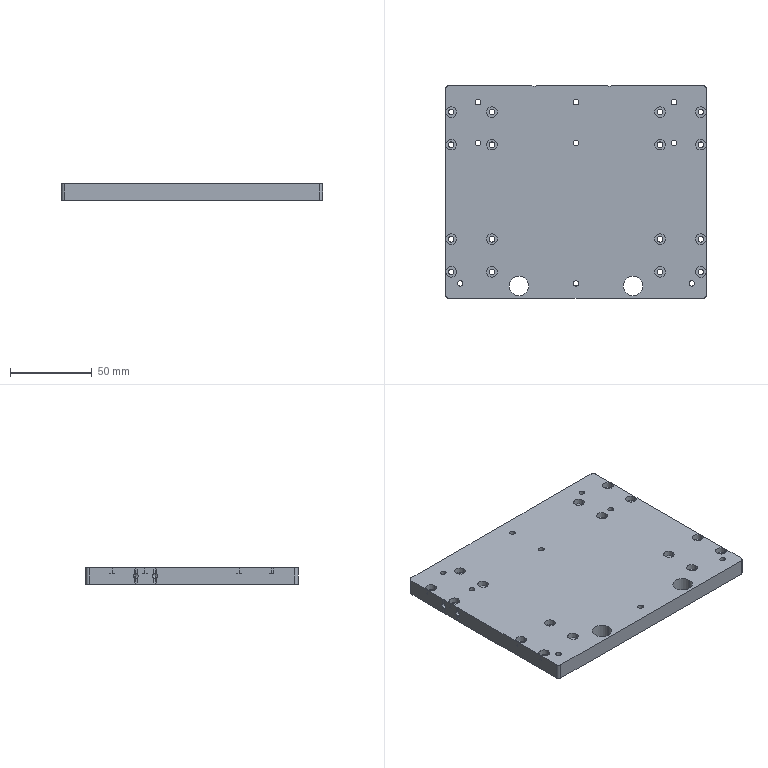Part | SolidWorks | features BaseBody 1 | 1 solid | 170 faces | box 160 x 130 x 10 mm | volume 201415 mm3 | cylinder 132 | plane 30 | cone 8 | commonest cylinder face diameters 3.4 x52 6.5 x36 4 x20 3.3 x14 10 x4 12 x4